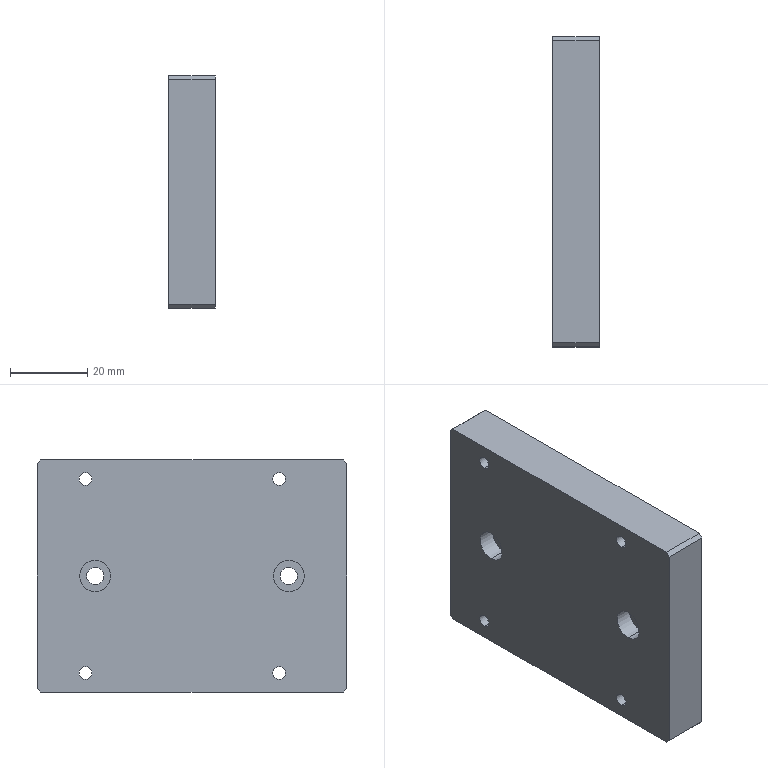Part | SolidWorks | features HoleWzd 2, Chamfer 1, Extrusion 1 | 1 solid | 28 faces | box 12 x 80 x 60 mm | volume 56468 mm3 | cylinder 16 | plane 12 | commonest cylinder face diameters 3.3 x8 4.5 x4 8 x4
STEP:
#1=CARTESIAN_POINT('',(4.6,-25.,-4.));
#2=VERTEX_POINT('',#1);
#3=CARTESIAN_POINT('',(4.6,-25.,4.));
#4=VERTEX_POINT('',#3);
#5=CARTESIAN_POINT('',(4.6,-25.,0.));
#6=DIRECTION('',(-1.,0.,0.));
#7=DIRECTION('',(0.,0.,1.));
#8=AXIS2_PLACEMENT_3D('',#5,#6,#7);
#9=CIRCLE('',#8,4.);
#10=EDGE_CURVE('',#2,#4,#9,.T.);
#11=ORIENTED_EDGE('',*,*,#10,.F.);
#12=CARTESIAN_POINT('',(0.,-25.,-4.));
#13=VERTEX_POINT('',#12);
#14=CARTESIAN_POINT('',(0.,-25.,-4.));
#15=DIRECTION('',(-1.,0.,0.));
#16=VECTOR('',#15,1000.);
#17=LINE('',#14,#16);
#18=EDGE_CURVE('',#2,#13,#17,.T.);
#19=ORIENTED_EDGE('',*,*,#18,.T.);
#20=CARTESIAN_POINT('',(0.,-25.,4.));
#21=VERTEX_POINT('',#20);
#22=CARTESIAN_POINT('',(0.,-25.,0.));
#23=DIRECTION('',(-1.,0.,0.));
#24=DIRECTION('',(0.,0.,1.));
#25=AXIS2_PLACEMENT_3D('',#22,#23,#24);
#26=CIRCLE('',#25,4.);
#27=EDGE_CURVE('',#13,#21,#26,.T.);
#28=ORIENTED_EDGE('',*,*,#27,.T.);
#29=CARTESIAN_POINT('',(0.,-25.,4.));
#30=DIRECTION('',(-1.,0.,0.));
#31=VECTOR('',#30,1000.);
#32=LINE('',#29,#31);
#33=EDGE_CURVE('',#4,#21,#32,.T.);
#34=ORIENTED_EDGE('',*,*,#33,.F.);
#35=EDGE_LOOP('',(#11,#19,#28,#34));
#36=FACE_OUTER_BOUND('',#35,.T.);
#37=CARTESIAN_POINT('',(0.,-25.,0.));
#38=DIRECTION('',(-1.,0.,0.));
#39=DIRECTION('',(0.,0.,1.));
#40=AXIS2_PLACEMENT_3D('',#37,#38,#39);
#41=CYLINDRICAL_SURFACE('',#40,4.);
#42=ADVANCED_FACE('',(#36),#41,.F.);
#43=CARTESIAN_POINT('',(12.,-25.,-2.25));
#44=VERTEX_POINT('',#43);
#45=CARTESIAN_POINT('',(12.,-25.,2.25));
#46=VERTEX_POINT('',#45);
#47=CARTESIAN_POINT('',(12.,-25.,0.));
#48=DIRECTION('',(-1.,0.,0.));
#49=DIRECTION('',(0.,0.,1.));
#50=AXIS2_PLACEMENT_3D('',#47,#48,#49);
#51=CIRCLE('',#50,2.25);
#52=EDGE_CURVE('',#44,#46,#51,.T.);
#53=ORIENTED_EDGE('',*,*,#52,.F.);
#54=CARTESIAN_POINT('',(4.6,-25.,-2.25));
#55=VERTEX_POINT('',#54);
#56=CARTESIAN_POINT('',(0.,-25.,-2.25));
#57=DIRECTION('',(-1.,0.,0.));
#58=VECTOR('',#57,1000.);
#59=LINE('',#56,#58);
#60=EDGE_CURVE('',#44,#55,#59,.T.);
#61=ORIENTED_EDGE('',*,*,#60,.T.);
#62=CARTESIAN_POINT('',(4.6,-25.,2.25));
#63=VERTEX_POINT('',#62);
#64=CARTESIAN_POINT('',(4.6,-25.,0.));
#65=DIRECTION('',(-1.,0.,0.));
#66=DIRECTION('',(0.,0.,1.));
#67=AXIS2_PLACEMENT_3D('',#64,#65,#66);
#68=CIRCLE('',#67,2.25);
#69=EDGE_CURVE('',#55,#63,#68,.T.);
#70=ORIENTED_EDGE('',*,*,#69,.T.);
#71=CARTESIAN_POINT('',(0.,-25.,2.25));
#72=DIRECTION('',(-1.,0.,0.));
#73=VECTOR('',#72,1000.);
#74=LINE('',#71,#73);
#75=EDGE_CURVE('',#46,#63,#74,.T.);
#76=ORIENTED_EDGE('',*,*,#75,.F.);
#77=EDGE_LOOP('',(#53,#61,#70,#76));
#78=FACE_OUTER_BOUND('',#77,.T.);
#79=CARTESIAN_POINT('',(0.,-25.,0.));
#80=DIRECTION('',(-1.,0.,0.));
#81=DIRECTION('',(0.,0.,1.));
#82=AXIS2_PLACEMENT_3D('',#79,#80,#81);
#83=CYLINDRICAL_SURFACE('',#82,2.25);
#84=ADVANCED_FACE('',(#78),#83,.F.);
#85=CARTESIAN_POINT('',(4.6,25.,-4.));
#86=VERTEX_POINT('',#85);
#87=CARTESIAN_POINT('',(4.6,25.,4.));
#88=VERTEX_POINT('',#87);
#89=CARTESIAN_POINT('',(4.6,25.,0.));
#90=DIRECTION('',(-1.,0.,0.));
#91=DIRECTION('',(0.,0.,1.));
#92=AXIS2_PLACEMENT_3D('',#89,#90,#91);
#93=CIRCLE('',#92,4.);
#94=EDGE_CURVE('',#86,#88,#93,.T.);
#95=ORIENTED_EDGE('',*,*,#94,.F.);
#96=CARTESIAN_POINT('',(0.,25.,-4.));
#97=VERTEX_POINT('',#96);
#98=CARTESIAN_POINT('',(0.,25.,-4.));
#99=DIRECTION('',(-1.,0.,0.));
#100=VECTOR('',#99,1000.);
#101=LINE('',#98,#100);
#102=EDGE_CURVE('',#86,#97,#101,.T.);
#103=ORIENTED_EDGE('',*,*,#102,.T.);
#104=CARTESIAN_POINT('',(0.,25.,4.));
#105=VERTEX_POINT('',#104);
#106=CARTESIAN_POINT('',(0.,25.,0.));
#107=DIRECTION('',(-1.,0.,0.));
#108=DIRECTION('',(0.,0.,1.));
#109=AXIS2_PLACEMENT_3D('',#106,#107,#108);
#110=CIRCLE('',#109,4.);
#111=EDGE_CURVE('',#97,#105,#110,.T.);
#112=ORIENTED_EDGE('',*,*,#111,.T.);
#113=CARTESIAN_POINT('',(0.,25.,4.));
#114=DIRECTION('',(-1.,0.,0.));
#115=VECTOR('',#114,1000.);
#116=LINE('',#113,#115);
#117=EDGE_CURVE('',#88,#105,#116,.T.);
#118=ORIENTED_EDGE('',*,*,#117,.F.);
#119=EDGE_LOOP('',(#95,#103,#112,#118));
#120=FACE_OUTER_BOUND('',#119,.T.);
#121=CARTESIAN_POINT('',(0.,25.,0.));
#122=DIRECTION('',(-1.,0.,0.));
#123=DIRECTION('',(0.,0.,1.));
#124=AXIS2_PLACEMENT_3D('',#121,#122,#123);
#125=CYLINDRICAL_SURFACE('',#124,4.);
#126=ADVANCED_FACE('',(#120),#125,.F.);
#127=CARTESIAN_POINT('',(12.,25.,-2.25));
#128=VERTEX_POINT('',#127);
#129=CARTESIAN_POINT('',(12.,25.,2.25));
#130=VERTEX_POINT('',#129);
#131=CARTESIAN_POINT('',(12.,25.,0.));
#132=DIRECTION('',(-1.,0.,0.));
#133=DIRECTION('',(0.,0.,1.));
#134=AXIS2_PLACEMENT_3D('',#131,#132,#133);
#135=CIRCLE('',#134,2.25);
#136=EDGE_CURVE('',#128,#130,#135,.T.);
#137=ORIENTED_EDGE('',*,*,#136,.F.);
#138=CARTESIAN_POINT('',(4.6,25.,-2.25));
#139=VERTEX_POINT('',#138);
#140=CARTESIAN_POINT('',(0.,25.,-2.25));
#141=DIRECTION('',(-1.,0.,0.));
#142=VECTOR('',#141,1000.);
#143=LINE('',#140,#142);
#144=EDGE_CURVE('',#128,#139,#143,.T.);
#145=ORIENTED_EDGE('',*,*,#144,.T.);
#146=CARTESIAN_POINT('',(4.6,25.,2.25));
#147=VERTEX_POINT('',#146);
#148=CARTESIAN_POINT('',(4.6,25.,0.));
#149=DIRECTION('',(-1.,0.,0.));
#150=DIRECTION('',(0.,0.,1.));
#151=AXIS2_PLACEMENT_3D('',#148,#149,#150);
#152=CIRCLE('',#151,2.25);
#153=EDGE_CURVE('',#139,#147,#152,.T.);
#154=ORIENTED_EDGE('',*,*,#153,.T.);
#155=CARTESIAN_POINT('',(0.,25.,2.25));
#156=DIRECTION('',(-1.,0.,0.));
#157=VECTOR('',#156,1000.);
#158=LINE('',#155,#157);
#159=EDGE_CURVE('',#130,#147,#158,.T.);
#160=ORIENTED_EDGE('',*,*,#159,.F.);
#161=EDGE_LOOP('',(#137,#145,#154,#160));
#162=FACE_OUTER_BOUND('',#161,.T.);
#163=CARTESIAN_POINT('',(0.,25.,0.));
#164=DIRECTION('',(-1.,0.,0.));
#165=DIRECTION('',(0.,0.,1.));
#166=AXIS2_PLACEMENT_3D('',#163,#164,#165);
#167=CYLINDRICAL_SURFACE('',#166,2.25);
#168=ADVANCED_FACE('',(#162),#167,.F.);
#169=CARTESIAN_POINT('',(12.,27.5,-26.65));
#170=VERTEX_POINT('',#169);
#171=CARTESIAN_POINT('',(12.,27.5,-23.35));
#172=VERTEX_POINT('',#171);
#173=CARTESIAN_POINT('',(12.,27.5,-25.));
#174=DIRECTION('',(-1.,0.,0.));
#175=DIRECTION('',(0.,0.,1.));
#176=AXIS2_PLACEMENT_3D('',#173,#174,#175);
#177=CIRCLE('',#176,1.65);
#178=EDGE_CURVE('',#170,#172,#177,.T.);
#179=ORIENTED_EDGE('',*,*,#178,.F.);
#180=CARTESIAN_POINT('',(0.,27.5,-26.65));
#181=VERTEX_POINT('',#180);
#182=CARTESIAN_POINT('',(0.,27.5,-26.65));
#183=DIRECTION('',(-1.,0.,0.));
#184=VECTOR('',#183,1000.);
#185=LINE('',#182,#184);
#186=EDGE_CURVE('',#170,#181,#185,.T.);
#187=ORIENTED_EDGE('',*,*,#186,.T.);
#188=CARTESIAN_POINT('',(0.,27.5,-23.35));
#189=VERTEX_POINT('',#188);
#190=CARTESIAN_POINT('',(0.,27.5,-25.));
#191=DIRECTION('',(-1.,0.,0.));
#192=DIRECTION('',(0.,0.,1.));
#193=AXIS2_PLACEMENT_3D('',#190,#191,#192);
#194=CIRCLE('',#193,1.65);
#195=EDGE_CURVE('',#181,#189,#194,.T.);
#196=ORIENTED_EDGE('',*,*,#195,.T.);
#197=CARTESIAN_POINT('',(0.,27.5,-23.35));
#198=DIRECTION('',(-1.,0.,0.));
#199=VECTOR('',#198,1000.);
#200=LINE('',#197,#199);
#201=EDGE_CURVE('',#172,#189,#200,.T.);
#202=ORIENTED_EDGE('',*,*,#201,.F.);
#203=EDGE_LOOP('',(#179,#187,#196,#202));
#204=FACE_OUTER_BOUND('',#203,.T.);
#205=CARTESIAN_POINT('',(0.,27.5,-25.));
#206=DIRECTION('',(-1.,0.,0.));
#207=DIRECTION('',(0.,0.,1.));
#208=AXIS2_PLACEMENT_3D('',#205,#206,#207);
#209=CYLINDRICAL_SURFACE('',#208,1.65);
#210=ADVANCED_FACE('',(#204),#209,.F.);
#211=CARTESIAN_POINT('',(12.,-22.5,-26.65));
#212=VERTEX_POINT('',#211);
#213=CARTESIAN_POINT('',(12.,-22.5,-23.35));
#214=VERTEX_POINT('',#213);
#215=CARTESIAN_POINT('',(12.,-22.5,-25.));
#216=DIRECTION('',(-1.,0.,0.));
#217=DIRECTION('',(0.,0.,1.));
#218=AXIS2_PLACEMENT_3D('',#215,#216,#217);
#219=CIRCLE('',#218,1.65);
#220=EDGE_CURVE('',#212,#214,#219,.T.);
#221=ORIENTED_EDGE('',*,*,#220,.F.);
#222=CARTESIAN_POINT('',(0.,-22.5,-26.65));
#223=VERTEX_POINT('',#222);
#224=CARTESIAN_POINT('',(0.,-22.5,-26.65));
#225=DIRECTION('',(-1.,0.,0.));
#226=VECTOR('',#225,1000.);
#227=LINE('',#224,#226);
#228=EDGE_CURVE('',#212,#223,#227,.T.);
#229=ORIENTED_EDGE('',*,*,#228,.T.);
#230=CARTESIAN_POINT('',(0.,-22.5,-23.35));
#231=VERTEX_POINT('',#230);
#232=CARTESIAN_POINT('',(0.,-22.5,-25.));
#233=DIRECTION('',(-1.,0.,0.));
#234=DIRECTION('',(0.,0.,1.));
#235=AXIS2_PLACEMENT_3D('',#232,#233,#234);
#236=CIRCLE('',#235,1.65);
#237=EDGE_CURVE('',#223,#231,#236,.T.);
#238=ORIENTED_EDGE('',*,*,#237,.T.);
#239=CARTESIAN_POINT('',(0.,-22.5,-23.35));
#240=DIRECTION('',(-1.,0.,0.));
#241=VECTOR('',#240,1000.);
#242=LINE('',#239,#241);
#243=EDGE_CURVE('',#214,#231,#242,.T.);
#244=ORIENTED_EDGE('',*,*,#243,.F.);
#245=EDGE_LOOP('',(#221,#229,#238,#244));
#246=FACE_OUTER_BOUND('',#245,.T.);
#247=CARTESIAN_POINT('',(0.,-22.5,-25.));
#248=DIRECTION('',(-1.,0.,0.));
#249=DIRECTION('',(0.,0.,1.));
#250=AXIS2_PLACEMENT_3D('',#247,#248,#249);
#251=CYLINDRICAL_SURFACE('',#250,1.65);
#252=ADVANCED_FACE('',(#246),#251,.F.);
#253=CARTESIAN_POINT('',(12.,-22.5,23.35));
#254=VERTEX_POINT('',#253);
#255=CARTESIAN_POINT('',(12.,-22.5,26.65));
#256=VERTEX_POINT('',#255);
#257=CARTESIAN_POINT('',(12.,-22.5,25.));
#258=DIRECTION('',(-1.,0.,0.));
#259=DIRECTION('',(0.,0.,1.));
#260=AXIS2_PLACEMENT_3D('',#257,#258,#259);
#261=CIRCLE('',#260,1.65);
#262=EDGE_CURVE('',#254,#256,#261,.T.);
#263=ORIENTED_EDGE('',*,*,#262,.F.);
#264=CARTESIAN_POINT('',(0.,-22.5,23.35));
#265=VERTEX_POINT('',#264);
#266=CARTESIAN_POINT('',(0.,-22.5,23.35));
#267=DIRECTION('',(-1.,0.,0.));
#268=VECTOR('',#267,1000.);
#269=LINE('',#266,#268);
#270=EDGE_CURVE('',#254,#265,#269,.T.);
#271=ORIENTED_EDGE('',*,*,#270,.T.);
#272=CARTESIAN_POINT('',(0.,-22.5,26.65));
#273=VERTEX_POINT('',#272);
#274=CARTESIAN_POINT('',(0.,-22.5,25.));
#275=DIRECTION('',(-1.,0.,0.));
#276=DIRECTION('',(0.,0.,1.));
#277=AXIS2_PLACEMENT_3D('',#274,#275,#276);
#278=CIRCLE('',#277,1.65);
#279=EDGE_CURVE('',#265,#273,#278,.T.);
#280=ORIENTED_EDGE('',*,*,#279,.T.);
#281=CARTESIAN_POINT('',(0.,-22.5,26.65));
#282=DIRECTION('',(-1.,0.,0.));
#283=VECTOR('',#282,1000.);
#284=LINE('',#281,#283);
#285=EDGE_CURVE('',#256,#273,#284,.T.);
#286=ORIENTED_EDGE('',*,*,#285,.F.);
#287=EDGE_LOOP('',(#263,#271,#280,#286));
#288=FACE_OUTER_BOUND('',#287,.T.);
#289=CARTESIAN_POINT('',(0.,-22.5,25.));
#290=DIRECTION('',(-1.,0.,0.));
#291=DIRECTION('',(0.,0.,1.));
#292=AXIS2_PLACEMENT_3D('',#289,#290,#291);
#293=CYLINDRICAL_SURFACE('',#292,1.65);
#294=ADVANCED_FACE('',(#288),#293,.F.);
#295=CARTESIAN_POINT('',(12.,27.5,23.35));
#296=VERTEX_POINT('',#295);
#297=CARTESIAN_POINT('',(12.,27.5,26.65));
#298=VERTEX_POINT('',#297);
#299=CARTESIAN_POINT('',(12.,27.5,25.));
#300=DIRECTION('',(-1.,0.,0.));
#301=DIRECTION('',(0.,0.,1.));
#302=AXIS2_PLACEMENT_3D('',#299,#300,#301);
#303=CIRCLE('',#302,1.65);
#304=EDGE_CURVE('',#296,#298,#303,.T.);
#305=ORIENTED_EDGE('',*,*,#304,.F.);
#306=CARTESIAN_POINT('',(0.,27.5,23.35));
#307=VERTEX_POINT('',#306);
#308=CARTESIAN_POINT('',(0.,27.5,23.35));
#309=DIRECTION('',(-1.,0.,0.));
#310=VECTOR('',#309,1000.);
#311=LINE('',#308,#310);
#312=EDGE_CURVE('',#296,#307,#311,.T.);
#313=ORIENTED_EDGE('',*,*,#312,.T.);
#314=CARTESIAN_POINT('',(0.,27.5,26.65));
#315=VERTEX_POINT('',#314);
#316=CARTESIAN_POINT('',(0.,27.5,25.));
#317=DIRECTION('',(-1.,0.,0.));
#318=DIRECTION('',(0.,0.,1.));
#319=AXIS2_PLACEMENT_3D('',#316,#317,#318);
#320=CIRCLE('',#319,1.65);
#321=EDGE_CURVE('',#307,#315,#320,.T.);
#322=ORIENTED_EDGE('',*,*,#321,.T.);
#323=CARTESIAN_POINT('',(0.,27.5,26.65));
#324=DIRECTION('',(-1.,0.,0.));
#325=VECTOR('',#324,1000.);
#326=LINE('',#323,#325);
#327=EDGE_CURVE('',#298,#315,#326,.T.);
#328=ORIENTED_EDGE('',*,*,#327,.F.);
#329=EDGE_LOOP('',(#305,#313,#322,#328));
#330=FACE_OUTER_BOUND('',#329,.T.);
#331=CARTESIAN_POINT('',(0.,27.5,25.));
#332=DIRECTION('',(-1.,0.,0.));
#333=DIRECTION('',(0.,0.,1.));
#334=AXIS2_PLACEMENT_3D('',#331,#332,#333);
#335=CYLINDRICAL_SURFACE('',#334,1.65);
#336=ADVANCED_FACE('',(#330),#335,.F.);
#337=CARTESIAN_POINT('',(12.,-39.,-30.));
#338=VERTEX_POINT('',#337);
#339=CARTESIAN_POINT('',(12.,39.,-30.));
#340=VERTEX_POINT('',#339);
#341=CARTESIAN_POINT('',(12.,-40.,-30.));
#342=DIRECTION('',(0.,1.,0.));
#343=VECTOR('',#342,1000.);
#344=LINE('',#341,#343);
#345=EDGE_CURVE('',#338,#340,#344,.T.);
#346=ORIENTED_EDGE('',*,*,#345,.F.);
#347=CARTESIAN_POINT('',(0.,-39.,-30.));
#348=VERTEX_POINT('',#347);
#349=CARTESIAN_POINT('',(12.,-39.,-30.));
#350=DIRECTION('',(-1.,0.,0.));
#351=VECTOR('',#350,1000.);
#352=LINE('',#349,#351);
#353=EDGE_CURVE('',#338,#348,#352,.T.);
#354=ORIENTED_EDGE('',*,*,#353,.T.);
#355=CARTESIAN_POINT('',(0.,39.,-30.));
#356=VERTEX_POINT('',#355);
#357=CARTESIAN_POINT('',(0.,-40.,-30.));
#358=DIRECTION('',(0.,1.,0.));
#359=VECTOR('',#358,1000.);
#360=LINE('',#357,#359);
#361=EDGE_CURVE('',#348,#356,#360,.T.);
#362=ORIENTED_EDGE('',*,*,#361,.T.);
#363=CARTESIAN_POINT('',(12.,39.,-30.));
#364=DIRECTION('',(1.,0.,0.));
#365=VECTOR('',#364,1000.);
#366=LINE('',#363,#365);
#367=EDGE_CURVE('',#356,#340,#366,.T.);
#368=ORIENTED_EDGE('',*,*,#367,.T.);
#369=EDGE_LOOP('',(#346,#354,#362,#368));
#370=FACE_OUTER_BOUND('',#369,.T.);
#371=CARTESIAN_POINT('',(12.,-40.,-30.));
#372=DIRECTION('',(0.,0.,1.));
#373=DIRECTION('',(1.,0.,0.));
#374=AXIS2_PLACEMENT_3D('',#371,#372,#373);
#375=PLANE('',#374);
#376=ADVANCED_FACE('',(#370),#375,.F.);
#377=CARTESIAN_POINT('',(12.,40.,-29.));
#378=VERTEX_POINT('',#377);
#379=CARTESIAN_POINT('',(12.,40.,29.));
#380=VERTEX_POINT('',#379);
#381=CARTESIAN_POINT('',(12.,40.,30.));
#382=DIRECTION('',(0.,0.,1.));
#383=VECTOR('',#382,1000.);
#384=LINE('',#381,#383);
#385=EDGE_CURVE('',#378,#380,#384,.T.);
#386=ORIENTED_EDGE('',*,*,#385,.F.);
#387=CARTESIAN_POINT('',(0.,40.,-29.));
#388=VERTEX_POINT('',#387);
#389=CARTESIAN_POINT('',(12.,40.,-29.));
#390=DIRECTION('',(-1.,0.,0.));
#391=VECTOR('',#390,1000.);
#392=LINE('',#389,#391);
#393=EDGE_CURVE('',#378,#388,#392,.T.);
#394=ORIENTED_EDGE('',*,*,#393,.T.);
#395=CARTESIAN_POINT('',(0.,40.,29.));
#396=VERTEX_POINT('',#395);
#397=CARTESIAN_POINT('',(0.,40.,30.));
#398=DIRECTION('',(0.,0.,1.));
#399=VECTOR('',#398,1000.);
#400=LINE('',#397,#399);
#401=EDGE_CURVE('',#388,#396,#400,.T.);
#402=ORIENTED_EDGE('',*,*,#401,.T.);
#403=CARTESIAN_POINT('',(12.,40.,29.));
#404=DIRECTION('',(1.,0.,0.));
#405=VECTOR('',#404,1000.);
#406=LINE('',#403,#405);
#407=EDGE_CURVE('',#396,#380,#406,.T.);
#408=ORIENTED_EDGE('',*,*,#407,.T.);
#409=EDGE_LOOP('',(#386,#394,#402,#408));
#410=FACE_OUTER_BOUND('',#409,.T.);
#411=CARTESIAN_POINT('',(12.,40.,30.));
#412=DIRECTION('',(0.,-1.,0.));
#413=DIRECTION('',(0.,0.,-1.));
#414=AXIS2_PLACEMENT_3D('',#411,#412,#413);
#415=PLANE('',#414);
#416=ADVANCED_FACE('',(#410),#415,.F.);
#417=CARTESIAN_POINT('',(0.,39.,30.));
#418=VERTEX_POINT('',#417);
#419=CARTESIAN_POINT('',(0.,-39.,30.));
#420=VERTEX_POINT('',#419);
#421=CARTESIAN_POINT('',(0.,-40.,30.));
#422=DIRECTION('',(0.,-1.,0.));
#423=VECTOR('',#422,1000.);
#424=LINE('',#421,#423);
#425=EDGE_CURVE('',#418,#420,#424,.T.);
#426=ORIENTED_EDGE('',*,*,#425,.T.);
#427=CARTESIAN_POINT('',(12.,-39.,30.));
#428=VERTEX_POINT('',#427);
#429=CARTESIAN_POINT('',(12.,-39.,30.));
#430=DIRECTION('',(1.,0.,0.));
#431=VECTOR('',#430,1000.);
#432=LINE('',#429,#431);
#433=EDGE_CURVE('',#420,#428,#432,.T.);
#434=ORIENTED_EDGE('',*,*,#433,.T.);
#435=CARTESIAN_POINT('',(12.,39.,30.));
#436=VERTEX_POINT('',#435);
#437=CARTESIAN_POINT('',(12.,-40.,30.));
#438=DIRECTION('',(0.,-1.,0.));
#439=VECTOR('',#438,1000.);
#440=LINE('',#437,#439);
#441=EDGE_CURVE('',#436,#428,#440,.T.);
#442=ORIENTED_EDGE('',*,*,#441,.F.);
#443=CARTESIAN_POINT('',(12.,39.,30.));
#444=DIRECTION('',(-1.,0.,0.));
#445=VECTOR('',#444,1000.);
#446=LINE('',#443,#445);
#447=EDGE_CURVE('',#436,#418,#446,.T.);
#448=ORIENTED_EDGE('',*,*,#447,.T.);
#449=EDGE_LOOP('',(#426,#434,#442,#448));
#450=FACE_OUTER_BOUND('',#449,.T.);
#451=CARTESIAN_POINT('',(12.,-40.,30.));
#452=DIRECTION('',(0.,0.,-1.));
#453=DIRECTION('',(-1.,0.,0.));
#454=AXIS2_PLACEMENT_3D('',#451,#452,#453);
#455=PLANE('',#454);
#456=ADVANCED_FACE('',(#450),#455,.F.);
#457=CARTESIAN_POINT('',(0.,-40.,29.));
#458=VERTEX_POINT('',#457);
#459=CARTESIAN_POINT('',(0.,-40.,-29.));
#460=VERTEX_POINT('',#459);
#461=CARTESIAN_POINT('',(0.,-40.,30.));
#462=DIRECTION('',(0.,0.,-1.));
#463=VECTOR('',#462,1000.);
#464=LINE('',#461,#463);
#465=EDGE_CURVE('',#458,#460,#464,.T.);
#466=ORIENTED_EDGE('',*,*,#465,.T.);
#467=CARTESIAN_POINT('',(12.,-40.,-29.));
#468=VERTEX_POINT('',#467);
#469=CARTESIAN_POINT('',(12.,-40.,-29.));
#470=DIRECTION('',(1.,0.,0.));
#471=VECTOR('',#470,1000.);
#472=LINE('',#469,#471);
#473=EDGE_CURVE('',#460,#468,#472,.T.);
#474=ORIENTED_EDGE('',*,*,#473,.T.);
#475=CARTESIAN_POINT('',(12.,-40.,29.));
#476=VERTEX_POINT('',#475);
#477=CARTESIAN_POINT('',(12.,-40.,30.));
#478=DIRECTION('',(0.,0.,-1.));
#479=VECTOR('',#478,1000.);
#480=LINE('',#477,#479);
#481=EDGE_CURVE('',#476,#468,#480,.T.);
#482=ORIENTED_EDGE('',*,*,#481,.F.);
#483=CARTESIAN_POINT('',(12.,-40.,29.));
#484=DIRECTION('',(-1.,0.,0.));
#485=VECTOR('',#484,1000.);
#486=LINE('',#483,#485);
#487=EDGE_CURVE('',#476,#458,#486,.T.);
#488=ORIENTED_EDGE('',*,*,#487,.T.);
#489=EDGE_LOOP('',(#466,#474,#482,#488));
#490=FACE_OUTER_BOUND('',#489,.T.);
#491=CARTESIAN_POINT('',(12.,-40.,30.));
#492=DIRECTION('',(0.,1.,0.));
#493=DIRECTION('',(0.,0.,1.));
#494=AXIS2_PLACEMENT_3D('',#491,#492,#493);
#495=PLANE('',#494);
#496=ADVANCED_FACE('',(#490),#495,.F.);
#497=CARTESIAN_POINT('',(12.,-25.,0.));
#498=DIRECTION('',(-1.,0.,0.));
#499=DIRECTION('',(0.,0.,1.));
#500=AXIS2_PLACEMENT_3D('',#497,#498,#499);
#501=CIRCLE('',#500,2.25);
#502=EDGE_CURVE('',#46,#44,#501,.T.);
#503=ORIENTED_EDGE('',*,*,#502,.T.);
#504=ORIENTED_EDGE('',*,*,#52,.T.);
#505=EDGE_LOOP('',(#503,#504));
#506=FACE_BOUND('',#505,.T.);
#507=CARTESIAN_POINT('',(12.,25.,0.));
#508=DIRECTION('',(-1.,0.,0.));
#509=DIRECTION('',(0.,0.,1.));
#510=AXIS2_PLACEMENT_3D('',#507,#508,#509);
#511=CIRCLE('',#510,2.25);
#512=EDGE_CURVE('',#130,#128,#511,.T.);
#513=ORIENTED_EDGE('',*,*,#512,.T.);
#514=ORIENTED_EDGE('',*,*,#136,.T.);
#515=EDGE_LOOP('',(#513,#514));
#516=FACE_BOUND('',#515,.T.);
#517=CARTESIAN_POINT('',(12.,27.5,-25.));
#518=DIRECTION('',(-1.,0.,0.));
#519=DIRECTION('',(0.,0.,1.));
#520=AXIS2_PLACEMENT_3D('',#517,#518,#519);
#521=CIRCLE('',#520,1.65);
#522=EDGE_CURVE('',#172,#170,#521,.T.);
#523=ORIENTED_EDGE('',*,*,#522,.T.);
#524=ORIENTED_EDGE('',*,*,#178,.T.);
#525=EDGE_LOOP('',(#523,#524));
#526=FACE_BOUND('',#525,.T.);
#527=CARTESIAN_POINT('',(12.,-22.5,-25.));
#528=DIRECTION('',(-1.,0.,0.));
#529=DIRECTION('',(0.,0.,1.));
#530=AXIS2_PLACEMENT_3D('',#527,#528,#529);
#531=CIRCLE('',#530,1.65);
#532=EDGE_CURVE('',#214,#212,#531,.T.);
#533=ORIENTED_EDGE('',*,*,#532,.T.);
#534=ORIENTED_EDGE('',*,*,#220,.T.);
#535=EDGE_LOOP('',(#533,#534));
#536=FACE_BOUND('',#535,.T.);
#537=CARTESIAN_POINT('',(12.,-22.5,25.));
#538=DIRECTION('',(-1.,0.,0.));
#539=DIRECTION('',(0.,0.,1.));
#540=AXIS2_PLACEMENT_3D('',#537,#538,#539);
#541=CIRCLE('',#540,1.65);
#542=EDGE_CURVE('',#256,#254,#541,.T.);
#543=ORIENTED_EDGE('',*,*,#542,.T.);
#544=ORIENTED_EDGE('',*,*,#262,.T.);
#545=EDGE_LOOP('',(#543,#544));
#546=FACE_BOUND('',#545,.T.);
#547=CARTESIAN_POINT('',(12.,27.5,25.));
#548=DIRECTION('',(-1.,0.,0.));
#549=DIRECTION('',(0.,0.,1.));
#550=AXIS2_PLACEMENT_3D('',#547,#548,#549);
#551=CIRCLE('',#550,1.65);
#552=EDGE_CURVE('',#298,#296,#551,.T.);
#553=ORIENTED_EDGE('',*,*,#552,.T.);
#554=ORIENTED_EDGE('',*,*,#304,.T.);
#555=EDGE_LOOP('',(#553,#554));
#556=FACE_BOUND('',#555,.T.);
#557=ORIENTED_EDGE('',*,*,#481,.T.);
#558=CARTESIAN_POINT('',(12.,-39.,-30.));
#559=DIRECTION('',(0.,0.7071,-0.7071));
#560=VECTOR('',#559,1000.);
#561=LINE('',#558,#560);
#562=EDGE_CURVE('',#468,#338,#561,.T.);
#563=ORIENTED_EDGE('',*,*,#562,.T.);
#564=ORIENTED_EDGE('',*,*,#345,.T.);
#565=CARTESIAN_POINT('',(12.,40.,-29.));
#566=DIRECTION('',(0.,0.7071,0.7071));
#567=VECTOR('',#566,1000.);
#568=LINE('',#565,#567);
#569=EDGE_CURVE('',#340,#378,#568,.T.);
#570=ORIENTED_EDGE('',*,*,#569,.T.);
#571=ORIENTED_EDGE('',*,*,#385,.T.);
#572=CARTESIAN_POINT('',(12.,39.,30.));
#573=DIRECTION('',(0.,-0.7071,0.7071));
#574=VECTOR('',#573,1000.);
#575=LINE('',#572,#574);
#576=EDGE_CURVE('',#380,#436,#575,.T.);
#577=ORIENTED_EDGE('',*,*,#576,.T.);
#578=ORIENTED_EDGE('',*,*,#441,.T.);
#579=CARTESIAN_POINT('',(12.,-40.,29.));
#580=DIRECTION('',(0.,-0.7071,-0.7071));
#581=VECTOR('',#580,1000.);
#582=LINE('',#579,#581);
#583=EDGE_CURVE('',#428,#476,#582,.T.);
#584=ORIENTED_EDGE('',*,*,#583,.T.);
#585=EDGE_LOOP('',(#557,#563,#564,#570,#571,#577,#578,#584));
#586=FACE_OUTER_BOUND('',#585,.T.);
#587=CARTESIAN_POINT('',(12.,0.,0.));
#588=DIRECTION('',(-1.,0.,0.));
#589=DIRECTION('',(0.,0.,1.));
#590=AXIS2_PLACEMENT_3D('',#587,#588,#589);
#591=PLANE('',#590);
#592=ADVANCED_FACE('',(#506,#516,#526,#536,#546,#556,#586),#591,.F.);
#593=CARTESIAN_POINT('',(0.,-25.,0.));
#594=DIRECTION('',(-1.,0.,0.));
#595=DIRECTION('',(0.,0.,1.));
#596=AXIS2_PLACEMENT_3D('',#593,#594,#595);
#597=CIRCLE('',#596,4.);
#598=EDGE_CURVE('',#21,#13,#597,.T.);
#599=ORIENTED_EDGE('',*,*,#598,.F.);
#600=ORIENTED_EDGE('',*,*,#27,.F.);
#601=EDGE_LOOP('',(#599,#600));
#602=FACE_BOUND('',#601,.T.);
#603=CARTESIAN_POINT('',(0.,25.,0.));
#604=DIRECTION('',(-1.,0.,0.));
#605=DIRECTION('',(0.,0.,1.));
#606=AXIS2_PLACEMENT_3D('',#603,#604,#605);
#607=CIRCLE('',#606,4.);
#608=EDGE_CURVE('',#105,#97,#607,.T.);
#609=ORIENTED_EDGE('',*,*,#608,.F.);
#610=ORIENTED_EDGE('',*,*,#111,.F.);
#611=EDGE_LOOP('',(#609,#610));
#612=FACE_BOUND('',#611,.T.);
#613=CARTESIAN_POINT('',(0.,27.5,-25.));
#614=DIRECTION('',(-1.,0.,0.));
#615=DIRECTION('',(0.,0.,1.));
#616=AXIS2_PLACEMENT_3D('',#613,#614,#615);
#617=CIRCLE('',#616,1.65);
#618=EDGE_CURVE('',#189,#181,#617,.T.);
#619=ORIENTED_EDGE('',*,*,#618,.F.);
#620=ORIENTED_EDGE('',*,*,#195,.F.);
#621=EDGE_LOOP('',(#619,#620));
#622=FACE_BOUND('',#621,.T.);
#623=CARTESIAN_POINT('',(0.,-22.5,-25.));
#624=DIRECTION('',(-1.,0.,0.));
#625=DIRECTION('',(0.,0.,1.));
#626=AXIS2_PLACEMENT_3D('',#623,#624,#625);
#627=CIRCLE('',#626,1.65);
#628=EDGE_CURVE('',#231,#223,#627,.T.);
#629=ORIENTED_EDGE('',*,*,#628,.F.);
#630=ORIENTED_EDGE('',*,*,#237,.F.);
#631=EDGE_LOOP('',(#629,#630));
#632=FACE_BOUND('',#631,.T.);
#633=CARTESIAN_POINT('',(0.,-22.5,25.));
#634=DIRECTION('',(-1.,0.,0.));
#635=DIRECTION('',(0.,0.,1.));
#636=AXIS2_PLACEMENT_3D('',#633,#634,#635);
#637=CIRCLE('',#636,1.65);
#638=EDGE_CURVE('',#273,#265,#637,.T.);
#639=ORIENTED_EDGE('',*,*,#638,.F.);
#640=ORIENTED_EDGE('',*,*,#279,.F.);
#641=EDGE_LOOP('',(#639,#640));
#642=FACE_BOUND('',#641,.T.);
#643=CARTESIAN_POINT('',(0.,27.5,25.));
#644=DIRECTION('',(-1.,0.,0.));
#645=DIRECTION('',(0.,0.,1.));
#646=AXIS2_PLACEMENT_3D('',#643,#644,#645);
#647=CIRCLE('',#646,1.65);
#648=EDGE_CURVE('',#315,#307,#647,.T.);
#649=ORIENTED_EDGE('',*,*,#648,.F.);
#650=ORIENTED_EDGE('',*,*,#321,.F.);
#651=EDGE_LOOP('',(#649,#650));
#652=FACE_BOUND('',#651,.T.);
#653=ORIENTED_EDGE('',*,*,#361,.F.);
#654=CARTESIAN_POINT('',(0.,-34.5,-34.5));
#655=DIRECTION('',(0.,-0.7071,0.7071));
#656=VECTOR('',#655,1000.);
#657=LINE('',#654,#656);
#658=EDGE_CURVE('',#348,#460,#657,.T.);
#659=ORIENTED_EDGE('',*,*,#658,.T.);
#660=ORIENTED_EDGE('',*,*,#465,.F.);
#661=CARTESIAN_POINT('',(0.,-34.5,34.5));
#662=DIRECTION('',(0.,0.7071,0.7071));
#663=VECTOR('',#662,1000.);
#664=LINE('',#661,#663);
#665=EDGE_CURVE('',#458,#420,#664,.T.);
#666=ORIENTED_EDGE('',*,*,#665,.T.);
#667=ORIENTED_EDGE('',*,*,#425,.F.);
#668=CARTESIAN_POINT('',(0.,34.5,34.5));
#669=DIRECTION('',(0.,0.7071,-0.7071));
#670=VECTOR('',#669,1000.);
#671=LINE('',#668,#670);
#672=EDGE_CURVE('',#418,#396,#671,.T.);
#673=ORIENTED_EDGE('',*,*,#672,.T.);
#674=ORIENTED_EDGE('',*,*,#401,.F.);
#675=CARTESIAN_POINT('',(0.,34.5,-34.5));
#676=DIRECTION('',(0.,-0.7071,-0.7071));
#677=VECTOR('',#676,1000.);
#678=LINE('',#675,#677);
#679=EDGE_CURVE('',#388,#356,#678,.T.);
#680=ORIENTED_EDGE('',*,*,#679,.T.);
#681=EDGE_LOOP('',(#653,#659,#660,#666,#667,#673,#674,#680));
#682=FACE_OUTER_BOUND('',#681,.T.);
#683=CARTESIAN_POINT('',(0.,0.,0.));
#684=DIRECTION('',(-1.,0.,0.));
#685=DIRECTION('',(0.,0.,1.));
#686=AXIS2_PLACEMENT_3D('',#683,#684,#685);
#687=PLANE('',#686);
#688=ADVANCED_FACE('',(#602,#612,#622,#632,#642,#652,#682),#687,.T.);
#689=ORIENTED_EDGE('',*,*,#312,.F.);
#690=ORIENTED_EDGE('',*,*,#552,.F.);
#691=ORIENTED_EDGE('',*,*,#327,.T.);
#692=ORIENTED_EDGE('',*,*,#648,.T.);
#693=EDGE_LOOP('',(#689,#690,#691,#692));
#694=FACE_OUTER_BOUND('',#693,.T.);
#695=CARTESIAN_POINT('',(0.,27.5,25.));
#696=DIRECTION('',(-1.,0.,0.));
#697=DIRECTION('',(0.,0.,1.));
#698=AXIS2_PLACEMENT_3D('',#695,#696,#697);
#699=CYLINDRICAL_SURFACE('',#698,1.65);
#700=ADVANCED_FACE('',(#694),#699,.F.);
#701=ORIENTED_EDGE('',*,*,#270,.F.);
#702=ORIENTED_EDGE('',*,*,#542,.F.);
#703=ORIENTED_EDGE('',*,*,#285,.T.);
#704=ORIENTED_EDGE('',*,*,#638,.T.);
#705=EDGE_LOOP('',(#701,#702,#703,#704));
#706=FACE_OUTER_BOUND('',#705,.T.);
#707=CARTESIAN_POINT('',(0.,-22.5,25.));
#708=DIRECTION('',(-1.,0.,0.));
#709=DIRECTION('',(0.,0.,1.));
#710=AXIS2_PLACEMENT_3D('',#707,#708,#709);
#711=CYLINDRICAL_SURFACE('',#710,1.65);
#712=ADVANCED_FACE('',(#706),#711,.F.);
#713=ORIENTED_EDGE('',*,*,#228,.F.);
#714=ORIENTED_EDGE('',*,*,#532,.F.);
#715=ORIENTED_EDGE('',*,*,#243,.T.);
#716=ORIENTED_EDGE('',*,*,#628,.T.);
#717=EDGE_LOOP('',(#713,#714,#715,#716));
#718=FACE_OUTER_BOUND('',#717,.T.);
#719=CARTESIAN_POINT('',(0.,-22.5,-25.));
#720=DIRECTION('',(-1.,0.,0.));
#721=DIRECTION('',(0.,0.,1.));
#722=AXIS2_PLACEMENT_3D('',#719,#720,#721);
#723=CYLINDRICAL_SURFACE('',#722,1.65);
#724=ADVANCED_FACE('',(#718),#723,.F.);
#725=ORIENTED_EDGE('',*,*,#186,.F.);
#726=ORIENTED_EDGE('',*,*,#522,.F.);
#727=ORIENTED_EDGE('',*,*,#201,.T.);
#728=ORIENTED_EDGE('',*,*,#618,.T.);
#729=EDGE_LOOP('',(#725,#726,#727,#728));
#730=FACE_OUTER_BOUND('',#729,.T.);
#731=CARTESIAN_POINT('',(0.,27.5,-25.));
#732=DIRECTION('',(-1.,0.,0.));
#733=DIRECTION('',(0.,0.,1.));
#734=AXIS2_PLACEMENT_3D('',#731,#732,#733);
#735=CYLINDRICAL_SURFACE('',#734,1.65);
#736=ADVANCED_FACE('',(#730),#735,.F.);
#737=ORIENTED_EDGE('',*,*,#144,.F.);
#738=ORIENTED_EDGE('',*,*,#512,.F.);
#739=ORIENTED_EDGE('',*,*,#159,.T.);
#740=CARTESIAN_POINT('',(4.6,25.,0.));
#741=DIRECTION('',(-1.,0.,0.));
#742=DIRECTION('',(0.,0.,1.));
#743=AXIS2_PLACEMENT_3D('',#740,#741,#742);
#744=CIRCLE('',#743,2.25);
#745=EDGE_CURVE('',#147,#139,#744,.T.);
#746=ORIENTED_EDGE('',*,*,#745,.T.);
#747=EDGE_LOOP('',(#737,#738,#739,#746));
#748=FACE_OUTER_BOUND('',#747,.T.);
#749=CARTESIAN_POINT('',(0.,25.,0.));
#750=DIRECTION('',(-1.,0.,0.));
#751=DIRECTION('',(0.,0.,1.));
#752=AXIS2_PLACEMENT_3D('',#749,#750,#751);
#753=CYLINDRICAL_SURFACE('',#752,2.25);
#754=ADVANCED_FACE('',(#748),#753,.F.);
#755=ORIENTED_EDGE('',*,*,#745,.F.);
#756=ORIENTED_EDGE('',*,*,#153,.F.);
#757=EDGE_LOOP('',(#755,#756));
#758=FACE_BOUND('',#757,.T.);
#759=CARTESIAN_POINT('',(4.6,25.,0.));
#760=DIRECTION('',(-1.,0.,0.));
#761=DIRECTION('',(0.,0.,1.));
#762=AXIS2_PLACEMENT_3D('',#759,#760,#761);
#763=CIRCLE('',#762,4.);
#764=EDGE_CURVE('',#88,#86,#763,.T.);
#765=ORIENTED_EDGE('',*,*,#764,.T.);
#766=ORIENTED_EDGE('',*,*,#94,.T.);
#767=EDGE_LOOP('',(#765,#766));
#768=FACE_OUTER_BOUND('',#767,.T.);
#769=CARTESIAN_POINT('',(4.6,27.25,0.));
#770=DIRECTION('',(1.,0.,0.));
#771=DIRECTION('',(0.,0.,-1.));
#772=AXIS2_PLACEMENT_3D('',#769,#770,#771);
#773=PLANE('',#772);
#774=ADVANCED_FACE('',(#758,#768),#773,.F.);
#775=ORIENTED_EDGE('',*,*,#102,.F.);
#776=ORIENTED_EDGE('',*,*,#764,.F.);
#777=ORIENTED_EDGE('',*,*,#117,.T.);
#778=ORIENTED_EDGE('',*,*,#608,.T.);
#779=EDGE_LOOP('',(#775,#776,#777,#778));
#780=FACE_OUTER_BOUND('',#779,.T.);
#781=CARTESIAN_POINT('',(0.,25.,0.));
#782=DIRECTION('',(-1.,0.,0.));
#783=DIRECTION('',(0.,0.,1.));
#784=AXIS2_PLACEMENT_3D('',#781,#782,#783);
#785=CYLINDRICAL_SURFACE('',#784,4.);
#786=ADVANCED_FACE('',(#780),#785,.F.);
#787=ORIENTED_EDGE('',*,*,#60,.F.);
#788=ORIENTED_EDGE('',*,*,#502,.F.);
#789=ORIENTED_EDGE('',*,*,#75,.T.);
#790=CARTESIAN_POINT('',(4.6,-25.,0.));
#791=DIRECTION('',(-1.,0.,0.));
#792=DIRECTION('',(0.,0.,1.));
#793=AXIS2_PLACEMENT_3D('',#790,#791,#792);
#794=CIRCLE('',#793,2.25);
#795=EDGE_CURVE('',#63,#55,#794,.T.);
#796=ORIENTED_EDGE('',*,*,#795,.T.);
#797=EDGE_LOOP('',(#787,#788,#789,#796));
#798=FACE_OUTER_BOUND('',#797,.T.);
#799=CARTESIAN_POINT('',(0.,-25.,0.));
#800=DIRECTION('',(-1.,0.,0.));
#801=DIRECTION('',(0.,0.,1.));
#802=AXIS2_PLACEMENT_3D('',#799,#800,#801);
#803=CYLINDRICAL_SURFACE('',#802,2.25);
#804=ADVANCED_FACE('',(#798),#803,.F.);
#805=ORIENTED_EDGE('',*,*,#795,.F.);
#806=ORIENTED_EDGE('',*,*,#69,.F.);
#807=EDGE_LOOP('',(#805,#806));
#808=FACE_BOUND('',#807,.T.);
#809=CARTESIAN_POINT('',(4.6,-25.,0.));
#810=DIRECTION('',(-1.,0.,0.));
#811=DIRECTION('',(0.,0.,1.));
#812=AXIS2_PLACEMENT_3D('',#809,#810,#811);
#813=CIRCLE('',#812,4.);
#814=EDGE_CURVE('',#4,#2,#813,.T.);
#815=ORIENTED_EDGE('',*,*,#814,.T.);
#816=ORIENTED_EDGE('',*,*,#10,.T.);
#817=EDGE_LOOP('',(#815,#816));
#818=FACE_OUTER_BOUND('',#817,.T.);
#819=CARTESIAN_POINT('',(4.6,-22.75,0.));
#820=DIRECTION('',(1.,0.,0.));
#821=DIRECTION('',(0.,0.,-1.));
#822=AXIS2_PLACEMENT_3D('',#819,#820,#821);
#823=PLANE('',#822);
#824=ADVANCED_FACE('',(#808,#818),#823,.F.);
#825=ORIENTED_EDGE('',*,*,#18,.F.);
#826=ORIENTED_EDGE('',*,*,#814,.F.);
#827=ORIENTED_EDGE('',*,*,#33,.T.);
#828=ORIENTED_EDGE('',*,*,#598,.T.);
#829=EDGE_LOOP('',(#825,#826,#827,#828));
#830=FACE_OUTER_BOUND('',#829,.T.);
#831=CARTESIAN_POINT('',(0.,-25.,0.));
#832=DIRECTION('',(-1.,0.,0.));
#833=DIRECTION('',(0.,0.,1.));
#834=AXIS2_PLACEMENT_3D('',#831,#832,#833);
#835=CYLINDRICAL_SURFACE('',#834,4.);
#836=ADVANCED_FACE('',(#830),#835,.F.);
#837=ORIENTED_EDGE('',*,*,#562,.F.);
#838=ORIENTED_EDGE('',*,*,#473,.F.);
#839=ORIENTED_EDGE('',*,*,#658,.F.);
#840=ORIENTED_EDGE('',*,*,#353,.F.);
#841=EDGE_LOOP('',(#837,#838,#839,#840));
#842=FACE_OUTER_BOUND('',#841,.T.);
#843=CARTESIAN_POINT('',(12.,-39.,-30.));
#844=DIRECTION('',(0.,0.7071,0.7071));
#845=DIRECTION('',(-1.,0.,0.));
#846=AXIS2_PLACEMENT_3D('',#843,#844,#845);
#847=PLANE('',#846);
#848=ADVANCED_FACE('',(#842),#847,.F.);
#849=ORIENTED_EDGE('',*,*,#569,.F.);
#850=ORIENTED_EDGE('',*,*,#367,.F.);
#851=ORIENTED_EDGE('',*,*,#679,.F.);
#852=ORIENTED_EDGE('',*,*,#393,.F.);
#853=EDGE_LOOP('',(#849,#850,#851,#852));
#854=FACE_OUTER_BOUND('',#853,.T.);
#855=CARTESIAN_POINT('',(12.,40.,-29.));
#856=DIRECTION('',(0.,-0.7071,0.7071));
#857=DIRECTION('',(-1.,0.,0.));
#858=AXIS2_PLACEMENT_3D('',#855,#856,#857);
#859=PLANE('',#858);
#860=ADVANCED_FACE('',(#854),#859,.F.);
#861=ORIENTED_EDGE('',*,*,#583,.F.);
#862=ORIENTED_EDGE('',*,*,#433,.F.);
#863=ORIENTED_EDGE('',*,*,#665,.F.);
#864=ORIENTED_EDGE('',*,*,#487,.F.);
#865=EDGE_LOOP('',(#861,#862,#863,#864));
#866=FACE_OUTER_BOUND('',#865,.T.);
#867=CARTESIAN_POINT('',(12.,-40.,29.));
#868=DIRECTION('',(0.,0.7071,-0.7071));
#869=DIRECTION('',(-1.,0.,0.));
#870=AXIS2_PLACEMENT_3D('',#867,#868,#869);
#871=PLANE('',#870);
#872=ADVANCED_FACE('',(#866),#871,.F.);
#873=ORIENTED_EDGE('',*,*,#576,.F.);
#874=ORIENTED_EDGE('',*,*,#407,.F.);
#875=ORIENTED_EDGE('',*,*,#672,.F.);
#876=ORIENTED_EDGE('',*,*,#447,.F.);
#877=EDGE_LOOP('',(#873,#874,#875,#876));
#878=FACE_OUTER_BOUND('',#877,.T.);
#879=CARTESIAN_POINT('',(12.,39.,30.));
#880=DIRECTION('',(0.,-0.7071,-0.7071));
#881=DIRECTION('',(-1.,0.,0.));
#882=AXIS2_PLACEMENT_3D('',#879,#880,#881);
#883=PLANE('',#882);
#884=ADVANCED_FACE('',(#878),#883,.F.);
#885=CLOSED_SHELL('',(#42,#84,#126,#168,#210,#252,#294,#336,#376,#416,#456,#496,#592,#688,#700,#712,#724,#736,#754,#774,#786,#804,#824,#836,#848,#860,#872,#884));
#886=MANIFOLD_SOLID_BREP('',#885);
#887=CARTESIAN_POINT('',(0.,0.,0.));
#888=DIRECTION('',(0.,0.,1.));
#889=DIRECTION('',(1.,0.,0.));
#890=AXIS2_PLACEMENT_3D('',#887,#888,#889);
#891=(LENGTH_UNIT()NAMED_UNIT(*)SI_UNIT(.MILLI.,.METRE.));
#892=UNCERTAINTY_MEASURE_WITH_UNIT(LENGTH_MEASURE(0.00001),#891,'','');
#893=(NAMED_UNIT(*)PLANE_ANGLE_UNIT()SI_UNIT($,.RADIAN.));
#894=(NAMED_UNIT(*)SI_UNIT($,.STERADIAN.)SOLID_ANGLE_UNIT());
#895=(GEOMETRIC_REPRESENTATION_CONTEXT(3)GLOBAL_UNCERTAINTY_ASSIGNED_CONTEXT((#892))GLOBAL_UNIT_ASSIGNED_CONTEXT((#891,#893,#894))REPRESENTATION_CONTEXT('',''));
#896=ADVANCED_BREP_SHAPE_REPRESENTATION('',(#886,#890),#895);